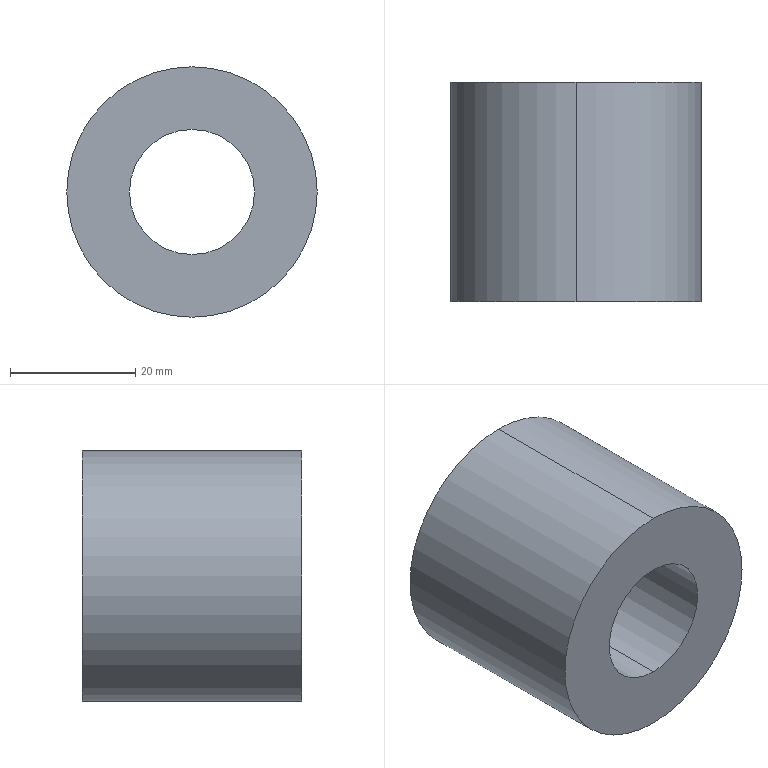Part | 1 solid | 6 faces | box 40 x 35 x 40 mm | volume 32987 mm3 | cylinder 4 | plane 2 | commonest cylinder face diameters 20 x2 40 x2
STEP:
#1=CARTESIAN_POINT('',(0.,0.,0.));
#2=DIRECTION('',(0.,0.,1.));
#3=DIRECTION('',(1.,0.,0.));
#4=AXIS2_PLACEMENT_3D('',#1,#2,#3);
#5=CARTESIAN_POINT('',(-239.028,4.5,-280.55));
#6=VERTEX_POINT('',#5);
#7=CARTESIAN_POINT('',(-239.028,4.5,-320.55));
#8=VERTEX_POINT('',#7);
#9=CARTESIAN_POINT('',(-239.028,4.5,-300.55));
#10=DIRECTION('',(0.,-1.,0.));
#11=DIRECTION('',(0.,0.,-1.));
#12=AXIS2_PLACEMENT_3D('',#9,#10,#11);
#13=CIRCLE('',#12,20.);
#14=CARTESIAN_POINT('',(-239.028,4.5,-300.55));
#15=DIRECTION('',(0.,1.,0.));
#16=DIRECTION('',(0.,0.,1.));
#17=AXIS2_PLACEMENT_3D('',#14,#15,#16);
#18=PLANE('',#17);
#19=CARTESIAN_POINT('',(-20.,0.));
#20=CARTESIAN_POINT('',(-20.,34.641));
#21=CARTESIAN_POINT('',(10.,17.321));
#22=CARTESIAN_POINT('',(40.,0.));
#23=CARTESIAN_POINT('',(10.,-17.321));
#24=CARTESIAN_POINT('',(-20.,-34.641));
#25=CARTESIAN_POINT('',(-20.,0.));
#26=(BOUNDED_CURVE()B_SPLINE_CURVE(2,(#19,#20,#21,#22,#23,#24,#25),.UNSPECIFIED.,.T.,.F.)B_SPLINE_CURVE_WITH_KNOTS((1,2,2,2,2,1),(-2.094,0.,2.094,4.189,6.283,8.378),.UNSPECIFIED.)CURVE()GEOMETRIC_REPRESENTATION_ITEM()RATIONAL_B_SPLINE_CURVE((1.,0.5,1.,0.5,1.,0.5,1.))REPRESENTATION_ITEM(''));
#27=(GEOMETRIC_REPRESENTATION_CONTEXT(2)PARAMETRIC_REPRESENTATION_CONTEXT()REPRESENTATION_CONTEXT('',''));
#28=DEFINITIONAL_REPRESENTATION('',(#26),#27);
#29=PCURVE('',#18,#28);
#30=CARTESIAN_POINT('',(-239.028,4.5,-300.55));
#31=DIRECTION('',(0.,-1.,0.));
#32=DIRECTION('',(1.,0.,0.));
#33=AXIS2_PLACEMENT_3D('',#30,#31,#32);
#34=CYLINDRICAL_SURFACE('',#33,20.);
#35=CARTESIAN_POINT('',(-1.571,0.));
#36=DIRECTION('',(1.,0.));
#37=VECTOR('',#36,1.);
#38=LINE('',#35,#37);
#39=(GEOMETRIC_REPRESENTATION_CONTEXT(2)PARAMETRIC_REPRESENTATION_CONTEXT()REPRESENTATION_CONTEXT('',''));
#40=DEFINITIONAL_REPRESENTATION('',(#38),#39);
#41=PCURVE('',#34,#40);
#42=SURFACE_CURVE('',#13,(#29,#41),.PCURVE_S1.);
#43=EDGE_CURVE('',#6,#8,#42,.T.);
#44=ORIENTED_EDGE('',*,*,#43,.F.);
#45=CARTESIAN_POINT('',(-239.028,4.5,-300.55));
#46=DIRECTION('',(0.,-1.,0.));
#47=DIRECTION('',(0.,0.,-1.));
#48=AXIS2_PLACEMENT_3D('',#45,#46,#47);
#49=CIRCLE('',#48,20.);
#50=CARTESIAN_POINT('',(-20.,0.));
#51=CARTESIAN_POINT('',(-20.,34.641));
#52=CARTESIAN_POINT('',(10.,17.321));
#53=CARTESIAN_POINT('',(40.,0.));
#54=CARTESIAN_POINT('',(10.,-17.321));
#55=CARTESIAN_POINT('',(-20.,-34.641));
#56=CARTESIAN_POINT('',(-20.,0.));
#57=(BOUNDED_CURVE()B_SPLINE_CURVE(2,(#50,#51,#52,#53,#54,#55,#56),.UNSPECIFIED.,.T.,.F.)B_SPLINE_CURVE_WITH_KNOTS((1,2,2,2,2,1),(-2.094,0.,2.094,4.189,6.283,8.378),.UNSPECIFIED.)CURVE()GEOMETRIC_REPRESENTATION_ITEM()RATIONAL_B_SPLINE_CURVE((1.,0.5,1.,0.5,1.,0.5,1.))REPRESENTATION_ITEM(''));
#58=(GEOMETRIC_REPRESENTATION_CONTEXT(2)PARAMETRIC_REPRESENTATION_CONTEXT()REPRESENTATION_CONTEXT('',''));
#59=DEFINITIONAL_REPRESENTATION('',(#57),#58);
#60=PCURVE('',#18,#59);
#61=CARTESIAN_POINT('',(-239.028,4.5,-300.55));
#62=DIRECTION('',(0.,-1.,0.));
#63=DIRECTION('',(-1.,0.,0.));
#64=AXIS2_PLACEMENT_3D('',#61,#62,#63);
#65=CYLINDRICAL_SURFACE('',#64,20.);
#66=CARTESIAN_POINT('',(1.571,0.));
#67=DIRECTION('',(1.,0.));
#68=VECTOR('',#67,1.);
#69=LINE('',#66,#68);
#70=(GEOMETRIC_REPRESENTATION_CONTEXT(2)PARAMETRIC_REPRESENTATION_CONTEXT()REPRESENTATION_CONTEXT('',''));
#71=DEFINITIONAL_REPRESENTATION('',(#69),#70);
#72=PCURVE('',#65,#71);
#73=SURFACE_CURVE('',#49,(#60,#72),.PCURVE_S1.);
#74=EDGE_CURVE('',#8,#6,#73,.T.);
#75=ORIENTED_EDGE('',*,*,#74,.F.);
#76=EDGE_LOOP('',(#44,#75));
#77=FACE_BOUND('',#76,.T.);
#78=CARTESIAN_POINT('',(-239.028,4.5,-310.55));
#79=VERTEX_POINT('',#78);
#80=CARTESIAN_POINT('',(-239.028,4.5,-290.55));
#81=VERTEX_POINT('',#80);
#82=CARTESIAN_POINT('',(-239.028,4.5,-300.55));
#83=DIRECTION('',(0.,-1.,0.));
#84=DIRECTION('',(0.,0.,-1.));
#85=AXIS2_PLACEMENT_3D('',#82,#83,#84);
#86=CIRCLE('',#85,10.);
#87=CARTESIAN_POINT('',(-10.,0.));
#88=CARTESIAN_POINT('',(-10.,17.321));
#89=CARTESIAN_POINT('',(5.,8.66));
#90=CARTESIAN_POINT('',(20.,0.));
#91=CARTESIAN_POINT('',(5.,-8.66));
#92=CARTESIAN_POINT('',(-10.,-17.321));
#93=CARTESIAN_POINT('',(-10.,0.));
#94=(BOUNDED_CURVE()B_SPLINE_CURVE(2,(#87,#88,#89,#90,#91,#92,#93),.UNSPECIFIED.,.T.,.F.)B_SPLINE_CURVE_WITH_KNOTS((1,2,2,2,2,1),(-2.094,0.,2.094,4.189,6.283,8.378),.UNSPECIFIED.)CURVE()GEOMETRIC_REPRESENTATION_ITEM()RATIONAL_B_SPLINE_CURVE((1.,0.5,1.,0.5,1.,0.5,1.))REPRESENTATION_ITEM(''));
#95=(GEOMETRIC_REPRESENTATION_CONTEXT(2)PARAMETRIC_REPRESENTATION_CONTEXT()REPRESENTATION_CONTEXT('',''));
#96=DEFINITIONAL_REPRESENTATION('',(#94),#95);
#97=PCURVE('',#18,#96);
#98=CARTESIAN_POINT('',(-239.028,4.5,-300.55));
#99=DIRECTION('',(0.,-1.,0.));
#100=DIRECTION('',(-1.,0.,0.));
#101=AXIS2_PLACEMENT_3D('',#98,#99,#100);
#102=CYLINDRICAL_SURFACE('',#101,10.);
#103=CARTESIAN_POINT('',(1.571,0.));
#104=DIRECTION('',(1.,0.));
#105=VECTOR('',#104,1.);
#106=LINE('',#103,#105);
#107=(GEOMETRIC_REPRESENTATION_CONTEXT(2)PARAMETRIC_REPRESENTATION_CONTEXT()REPRESENTATION_CONTEXT('',''));
#108=DEFINITIONAL_REPRESENTATION('',(#106),#107);
#109=PCURVE('',#102,#108);
#110=SURFACE_CURVE('',#86,(#97,#109),.PCURVE_S1.);
#111=EDGE_CURVE('',#79,#81,#110,.T.);
#112=ORIENTED_EDGE('',*,*,#111,.T.);
#113=CARTESIAN_POINT('',(-239.028,4.5,-300.55));
#114=DIRECTION('',(0.,-1.,0.));
#115=DIRECTION('',(0.,0.,-1.));
#116=AXIS2_PLACEMENT_3D('',#113,#114,#115);
#117=CIRCLE('',#116,10.);
#118=CARTESIAN_POINT('',(-10.,0.));
#119=CARTESIAN_POINT('',(-10.,17.321));
#120=CARTESIAN_POINT('',(5.,8.66));
#121=CARTESIAN_POINT('',(20.,0.));
#122=CARTESIAN_POINT('',(5.,-8.66));
#123=CARTESIAN_POINT('',(-10.,-17.321));
#124=CARTESIAN_POINT('',(-10.,0.));
#125=(BOUNDED_CURVE()B_SPLINE_CURVE(2,(#118,#119,#120,#121,#122,#123,#124),.UNSPECIFIED.,.T.,.F.)B_SPLINE_CURVE_WITH_KNOTS((1,2,2,2,2,1),(-2.094,0.,2.094,4.189,6.283,8.378),.UNSPECIFIED.)CURVE()GEOMETRIC_REPRESENTATION_ITEM()RATIONAL_B_SPLINE_CURVE((1.,0.5,1.,0.5,1.,0.5,1.))REPRESENTATION_ITEM(''));
#126=(GEOMETRIC_REPRESENTATION_CONTEXT(2)PARAMETRIC_REPRESENTATION_CONTEXT()REPRESENTATION_CONTEXT('',''));
#127=DEFINITIONAL_REPRESENTATION('',(#125),#126);
#128=PCURVE('',#18,#127);
#129=CARTESIAN_POINT('',(-239.028,4.5,-300.55));
#130=DIRECTION('',(0.,-1.,0.));
#131=DIRECTION('',(1.,0.,0.));
#132=AXIS2_PLACEMENT_3D('',#129,#130,#131);
#133=CYLINDRICAL_SURFACE('',#132,10.);
#134=CARTESIAN_POINT('',(-1.571,0.));
#135=DIRECTION('',(1.,0.));
#136=VECTOR('',#135,1.);
#137=LINE('',#134,#136);
#138=(GEOMETRIC_REPRESENTATION_CONTEXT(2)PARAMETRIC_REPRESENTATION_CONTEXT()REPRESENTATION_CONTEXT('',''));
#139=DEFINITIONAL_REPRESENTATION('',(#137),#138);
#140=PCURVE('',#133,#139);
#141=SURFACE_CURVE('',#117,(#128,#140),.PCURVE_S1.);
#142=EDGE_CURVE('',#81,#79,#141,.T.);
#143=ORIENTED_EDGE('',*,*,#142,.T.);
#144=EDGE_LOOP('',(#112,#143));
#145=FACE_BOUND('',#144,.T.);
#146=ADVANCED_FACE('',(#77,#145),#18,.T.);
#147=ORIENTED_EDGE('',*,*,#142,.T.);
#148=CARTESIAN_POINT('',(-239.028,-30.5,-310.55));
#149=VERTEX_POINT('',#148);
#150=CARTESIAN_POINT('',(-239.028,4.5,-310.55));
#151=DIRECTION('',(0.,-1.,0.));
#152=VECTOR('',#151,1.);
#153=LINE('',#150,#152);
#154=CARTESIAN_POINT('',(4.712,0.));
#155=DIRECTION('',(0.,1.));
#156=VECTOR('',#155,1.);
#157=LINE('',#154,#156);
#158=(GEOMETRIC_REPRESENTATION_CONTEXT(2)PARAMETRIC_REPRESENTATION_CONTEXT()REPRESENTATION_CONTEXT('',''));
#159=DEFINITIONAL_REPRESENTATION('',(#157),#158);
#160=PCURVE('',#133,#159);
#161=CARTESIAN_POINT('',(1.571,0.));
#162=DIRECTION('',(0.,1.));
#163=VECTOR('',#162,1.);
#164=LINE('',#161,#163);
#165=(GEOMETRIC_REPRESENTATION_CONTEXT(2)PARAMETRIC_REPRESENTATION_CONTEXT()REPRESENTATION_CONTEXT('',''));
#166=DEFINITIONAL_REPRESENTATION('',(#164),#165);
#167=PCURVE('',#102,#166);
#168=SURFACE_CURVE('',#153,(#160,#167),.PCURVE_S1.);
#169=EDGE_CURVE('',#79,#149,#168,.T.);
#170=ORIENTED_EDGE('',*,*,#169,.T.);
#171=CARTESIAN_POINT('',(-239.028,-30.5,-290.55));
#172=VERTEX_POINT('',#171);
#173=CARTESIAN_POINT('',(-239.028,-30.5,-300.55));
#174=DIRECTION('',(0.,-1.,0.));
#175=DIRECTION('',(0.,0.,-1.));
#176=AXIS2_PLACEMENT_3D('',#173,#174,#175);
#177=CIRCLE('',#176,10.);
#178=CARTESIAN_POINT('',(-1.571,35.));
#179=DIRECTION('',(1.,0.));
#180=VECTOR('',#179,1.);
#181=LINE('',#178,#180);
#182=(GEOMETRIC_REPRESENTATION_CONTEXT(2)PARAMETRIC_REPRESENTATION_CONTEXT()REPRESENTATION_CONTEXT('',''));
#183=DEFINITIONAL_REPRESENTATION('',(#181),#182);
#184=PCURVE('',#133,#183);
#185=CARTESIAN_POINT('',(-239.028,-30.5,-300.55));
#186=DIRECTION('',(0.,1.,0.));
#187=DIRECTION('',(0.,0.,1.));
#188=AXIS2_PLACEMENT_3D('',#185,#186,#187);
#189=PLANE('',#188);
#190=CARTESIAN_POINT('',(-10.,0.));
#191=CARTESIAN_POINT('',(-10.,17.321));
#192=CARTESIAN_POINT('',(5.,8.66));
#193=CARTESIAN_POINT('',(20.,0.));
#194=CARTESIAN_POINT('',(5.,-8.66));
#195=CARTESIAN_POINT('',(-10.,-17.321));
#196=CARTESIAN_POINT('',(-10.,0.));
#197=(BOUNDED_CURVE()B_SPLINE_CURVE(2,(#190,#191,#192,#193,#194,#195,#196),.UNSPECIFIED.,.T.,.F.)B_SPLINE_CURVE_WITH_KNOTS((1,2,2,2,2,1),(-2.094,0.,2.094,4.189,6.283,8.378),.UNSPECIFIED.)CURVE()GEOMETRIC_REPRESENTATION_ITEM()RATIONAL_B_SPLINE_CURVE((1.,0.5,1.,0.5,1.,0.5,1.))REPRESENTATION_ITEM(''));
#198=(GEOMETRIC_REPRESENTATION_CONTEXT(2)PARAMETRIC_REPRESENTATION_CONTEXT()REPRESENTATION_CONTEXT('',''));
#199=DEFINITIONAL_REPRESENTATION('',(#197),#198);
#200=PCURVE('',#189,#199);
#201=SURFACE_CURVE('',#177,(#184,#200),.PCURVE_S1.);
#202=EDGE_CURVE('',#172,#149,#201,.T.);
#203=ORIENTED_EDGE('',*,*,#202,.F.);
#204=CARTESIAN_POINT('',(-239.028,4.5,-290.55));
#205=DIRECTION('',(0.,-1.,0.));
#206=VECTOR('',#205,1.);
#207=LINE('',#204,#206);
#208=CARTESIAN_POINT('',(1.571,0.));
#209=DIRECTION('',(0.,1.));
#210=VECTOR('',#209,1.);
#211=LINE('',#208,#210);
#212=(GEOMETRIC_REPRESENTATION_CONTEXT(2)PARAMETRIC_REPRESENTATION_CONTEXT()REPRESENTATION_CONTEXT('',''));
#213=DEFINITIONAL_REPRESENTATION('',(#211),#212);
#214=PCURVE('',#133,#213);
#215=CARTESIAN_POINT('',(4.712,0.));
#216=DIRECTION('',(0.,1.));
#217=VECTOR('',#216,1.);
#218=LINE('',#215,#217);
#219=(GEOMETRIC_REPRESENTATION_CONTEXT(2)PARAMETRIC_REPRESENTATION_CONTEXT()REPRESENTATION_CONTEXT('',''));
#220=DEFINITIONAL_REPRESENTATION('',(#218),#219);
#221=PCURVE('',#102,#220);
#222=SURFACE_CURVE('',#207,(#214,#221),.PCURVE_S1.);
#223=EDGE_CURVE('',#81,#172,#222,.T.);
#224=ORIENTED_EDGE('',*,*,#223,.F.);
#225=EDGE_LOOP('',(#147,#170,#203,#224));
#226=FACE_BOUND('',#225,.F.);
#227=ADVANCED_FACE('',(#226),#133,.F.);
#228=CARTESIAN_POINT('',(-239.028,-30.5,-320.55));
#229=VERTEX_POINT('',#228);
#230=CARTESIAN_POINT('',(-239.028,-30.5,-280.55));
#231=VERTEX_POINT('',#230);
#232=CARTESIAN_POINT('',(-239.028,-30.5,-300.55));
#233=DIRECTION('',(0.,-1.,0.));
#234=DIRECTION('',(0.,0.,-1.));
#235=AXIS2_PLACEMENT_3D('',#232,#233,#234);
#236=CIRCLE('',#235,20.);
#237=CARTESIAN_POINT('',(-20.,0.));
#238=CARTESIAN_POINT('',(-20.,34.641));
#239=CARTESIAN_POINT('',(10.,17.321));
#240=CARTESIAN_POINT('',(40.,0.));
#241=CARTESIAN_POINT('',(10.,-17.321));
#242=CARTESIAN_POINT('',(-20.,-34.641));
#243=CARTESIAN_POINT('',(-20.,0.));
#244=(BOUNDED_CURVE()B_SPLINE_CURVE(2,(#237,#238,#239,#240,#241,#242,#243),.UNSPECIFIED.,.T.,.F.)B_SPLINE_CURVE_WITH_KNOTS((1,2,2,2,2,1),(-2.094,0.,2.094,4.189,6.283,8.378),.UNSPECIFIED.)CURVE()GEOMETRIC_REPRESENTATION_ITEM()RATIONAL_B_SPLINE_CURVE((1.,0.5,1.,0.5,1.,0.5,1.))REPRESENTATION_ITEM(''));
#245=(GEOMETRIC_REPRESENTATION_CONTEXT(2)PARAMETRIC_REPRESENTATION_CONTEXT()REPRESENTATION_CONTEXT('',''));
#246=DEFINITIONAL_REPRESENTATION('',(#244),#245);
#247=PCURVE('',#189,#246);
#248=CARTESIAN_POINT('',(1.571,35.));
#249=DIRECTION('',(1.,0.));
#250=VECTOR('',#249,1.);
#251=LINE('',#248,#250);
#252=(GEOMETRIC_REPRESENTATION_CONTEXT(2)PARAMETRIC_REPRESENTATION_CONTEXT()REPRESENTATION_CONTEXT('',''));
#253=DEFINITIONAL_REPRESENTATION('',(#251),#252);
#254=PCURVE('',#65,#253);
#255=SURFACE_CURVE('',#236,(#247,#254),.PCURVE_S1.);
#256=EDGE_CURVE('',#229,#231,#255,.T.);
#257=ORIENTED_EDGE('',*,*,#256,.T.);
#258=CARTESIAN_POINT('',(-239.028,-30.5,-300.55));
#259=DIRECTION('',(0.,-1.,0.));
#260=DIRECTION('',(0.,0.,-1.));
#261=AXIS2_PLACEMENT_3D('',#258,#259,#260);
#262=CIRCLE('',#261,20.);
#263=CARTESIAN_POINT('',(-20.,0.));
#264=CARTESIAN_POINT('',(-20.,34.641));
#265=CARTESIAN_POINT('',(10.,17.321));
#266=CARTESIAN_POINT('',(40.,0.));
#267=CARTESIAN_POINT('',(10.,-17.321));
#268=CARTESIAN_POINT('',(-20.,-34.641));
#269=CARTESIAN_POINT('',(-20.,0.));
#270=(BOUNDED_CURVE()B_SPLINE_CURVE(2,(#263,#264,#265,#266,#267,#268,#269),.UNSPECIFIED.,.T.,.F.)B_SPLINE_CURVE_WITH_KNOTS((1,2,2,2,2,1),(-2.094,0.,2.094,4.189,6.283,8.378),.UNSPECIFIED.)CURVE()GEOMETRIC_REPRESENTATION_ITEM()RATIONAL_B_SPLINE_CURVE((1.,0.5,1.,0.5,1.,0.5,1.))REPRESENTATION_ITEM(''));
#271=(GEOMETRIC_REPRESENTATION_CONTEXT(2)PARAMETRIC_REPRESENTATION_CONTEXT()REPRESENTATION_CONTEXT('',''));
#272=DEFINITIONAL_REPRESENTATION('',(#270),#271);
#273=PCURVE('',#189,#272);
#274=CARTESIAN_POINT('',(-1.571,35.));
#275=DIRECTION('',(1.,0.));
#276=VECTOR('',#275,1.);
#277=LINE('',#274,#276);
#278=(GEOMETRIC_REPRESENTATION_CONTEXT(2)PARAMETRIC_REPRESENTATION_CONTEXT()REPRESENTATION_CONTEXT('',''));
#279=DEFINITIONAL_REPRESENTATION('',(#277),#278);
#280=PCURVE('',#34,#279);
#281=SURFACE_CURVE('',#262,(#273,#280),.PCURVE_S1.);
#282=EDGE_CURVE('',#231,#229,#281,.T.);
#283=ORIENTED_EDGE('',*,*,#282,.T.);
#284=EDGE_LOOP('',(#257,#283));
#285=FACE_BOUND('',#284,.T.);
#286=ORIENTED_EDGE('',*,*,#202,.F.);
#287=CARTESIAN_POINT('',(-239.028,-30.5,-300.55));
#288=DIRECTION('',(0.,-1.,0.));
#289=DIRECTION('',(0.,0.,-1.));
#290=AXIS2_PLACEMENT_3D('',#287,#288,#289);
#291=CIRCLE('',#290,10.);
#292=CARTESIAN_POINT('',(-10.,0.));
#293=CARTESIAN_POINT('',(-10.,17.321));
#294=CARTESIAN_POINT('',(5.,8.66));
#295=CARTESIAN_POINT('',(20.,0.));
#296=CARTESIAN_POINT('',(5.,-8.66));
#297=CARTESIAN_POINT('',(-10.,-17.321));
#298=CARTESIAN_POINT('',(-10.,0.));
#299=(BOUNDED_CURVE()B_SPLINE_CURVE(2,(#292,#293,#294,#295,#296,#297,#298),.UNSPECIFIED.,.T.,.F.)B_SPLINE_CURVE_WITH_KNOTS((1,2,2,2,2,1),(-2.094,0.,2.094,4.189,6.283,8.378),.UNSPECIFIED.)CURVE()GEOMETRIC_REPRESENTATION_ITEM()RATIONAL_B_SPLINE_CURVE((1.,0.5,1.,0.5,1.,0.5,1.))REPRESENTATION_ITEM(''));
#300=(GEOMETRIC_REPRESENTATION_CONTEXT(2)PARAMETRIC_REPRESENTATION_CONTEXT()REPRESENTATION_CONTEXT('',''));
#301=DEFINITIONAL_REPRESENTATION('',(#299),#300);
#302=PCURVE('',#189,#301);
#303=CARTESIAN_POINT('',(1.571,35.));
#304=DIRECTION('',(1.,0.));
#305=VECTOR('',#304,1.);
#306=LINE('',#303,#305);
#307=(GEOMETRIC_REPRESENTATION_CONTEXT(2)PARAMETRIC_REPRESENTATION_CONTEXT()REPRESENTATION_CONTEXT('',''));
#308=DEFINITIONAL_REPRESENTATION('',(#306),#307);
#309=PCURVE('',#102,#308);
#310=SURFACE_CURVE('',#291,(#302,#309),.PCURVE_S1.);
#311=EDGE_CURVE('',#149,#172,#310,.T.);
#312=ORIENTED_EDGE('',*,*,#311,.F.);
#313=EDGE_LOOP('',(#286,#312));
#314=FACE_BOUND('',#313,.T.);
#315=ADVANCED_FACE('',(#285,#314),#189,.F.);
#316=CARTESIAN_POINT('',(-239.028,4.5,-280.55));
#317=DIRECTION('',(0.,-1.,0.));
#318=VECTOR('',#317,1.);
#319=LINE('',#316,#318);
#320=CARTESIAN_POINT('',(1.571,0.));
#321=DIRECTION('',(0.,1.));
#322=VECTOR('',#321,1.);
#323=LINE('',#320,#322);
#324=(GEOMETRIC_REPRESENTATION_CONTEXT(2)PARAMETRIC_REPRESENTATION_CONTEXT()REPRESENTATION_CONTEXT('',''));
#325=DEFINITIONAL_REPRESENTATION('',(#323),#324);
#326=PCURVE('',#34,#325);
#327=CARTESIAN_POINT('',(4.712,0.));
#328=DIRECTION('',(0.,1.));
#329=VECTOR('',#328,1.);
#330=LINE('',#327,#329);
#331=(GEOMETRIC_REPRESENTATION_CONTEXT(2)PARAMETRIC_REPRESENTATION_CONTEXT()REPRESENTATION_CONTEXT('',''));
#332=DEFINITIONAL_REPRESENTATION('',(#330),#331);
#333=PCURVE('',#65,#332);
#334=SURFACE_CURVE('',#319,(#326,#333),.PCURVE_S1.);
#335=EDGE_CURVE('',#6,#231,#334,.T.);
#336=ORIENTED_EDGE('',*,*,#335,.F.);
#337=ORIENTED_EDGE('',*,*,#43,.T.);
#338=CARTESIAN_POINT('',(-239.028,4.5,-320.55));
#339=DIRECTION('',(0.,-1.,0.));
#340=VECTOR('',#339,1.);
#341=LINE('',#338,#340);
#342=CARTESIAN_POINT('',(4.712,0.));
#343=DIRECTION('',(0.,1.));
#344=VECTOR('',#343,1.);
#345=LINE('',#342,#344);
#346=(GEOMETRIC_REPRESENTATION_CONTEXT(2)PARAMETRIC_REPRESENTATION_CONTEXT()REPRESENTATION_CONTEXT('',''));
#347=DEFINITIONAL_REPRESENTATION('',(#345),#346);
#348=PCURVE('',#34,#347);
#349=CARTESIAN_POINT('',(1.571,0.));
#350=DIRECTION('',(0.,1.));
#351=VECTOR('',#350,1.);
#352=LINE('',#349,#351);
#353=(GEOMETRIC_REPRESENTATION_CONTEXT(2)PARAMETRIC_REPRESENTATION_CONTEXT()REPRESENTATION_CONTEXT('',''));
#354=DEFINITIONAL_REPRESENTATION('',(#352),#353);
#355=PCURVE('',#65,#354);
#356=SURFACE_CURVE('',#341,(#348,#355),.PCURVE_S1.);
#357=EDGE_CURVE('',#8,#229,#356,.T.);
#358=ORIENTED_EDGE('',*,*,#357,.T.);
#359=ORIENTED_EDGE('',*,*,#282,.F.);
#360=EDGE_LOOP('',(#336,#337,#358,#359));
#361=FACE_BOUND('',#360,.T.);
#362=ADVANCED_FACE('',(#361),#34,.T.);
#363=ORIENTED_EDGE('',*,*,#311,.F.);
#364=ORIENTED_EDGE('',*,*,#169,.F.);
#365=ORIENTED_EDGE('',*,*,#111,.T.);
#366=ORIENTED_EDGE('',*,*,#223,.T.);
#367=EDGE_LOOP('',(#363,#364,#365,#366));
#368=FACE_BOUND('',#367,.F.);
#369=ADVANCED_FACE('',(#368),#102,.F.);
#370=ORIENTED_EDGE('',*,*,#335,.T.);
#371=ORIENTED_EDGE('',*,*,#256,.F.);
#372=ORIENTED_EDGE('',*,*,#357,.F.);
#373=ORIENTED_EDGE('',*,*,#74,.T.);
#374=EDGE_LOOP('',(#370,#371,#372,#373));
#375=FACE_BOUND('',#374,.T.);
#376=ADVANCED_FACE('',(#375),#65,.T.);
#377=CLOSED_SHELL('',(#146,#227,#315,#362,#369,#376));
#378=MANIFOLD_SOLID_BREP('',#377);
#379=(LENGTH_UNIT()NAMED_UNIT(*)SI_UNIT(.MILLI.,.METRE.));
#380=UNCERTAINTY_MEASURE_WITH_UNIT(LENGTH_MEASURE(0.0000001),#379,'','');
#381=(NAMED_UNIT(*)PLANE_ANGLE_UNIT()SI_UNIT($,.RADIAN.));
#382=(NAMED_UNIT(*)SI_UNIT($,.STERADIAN.)SOLID_ANGLE_UNIT());
#383=(GEOMETRIC_REPRESENTATION_CONTEXT(3)GLOBAL_UNCERTAINTY_ASSIGNED_CONTEXT((#380))GLOBAL_UNIT_ASSIGNED_CONTEXT((#379,#381,#382))REPRESENTATION_CONTEXT('',''));
#384=ADVANCED_BREP_SHAPE_REPRESENTATION('',(#4,#378),#383);